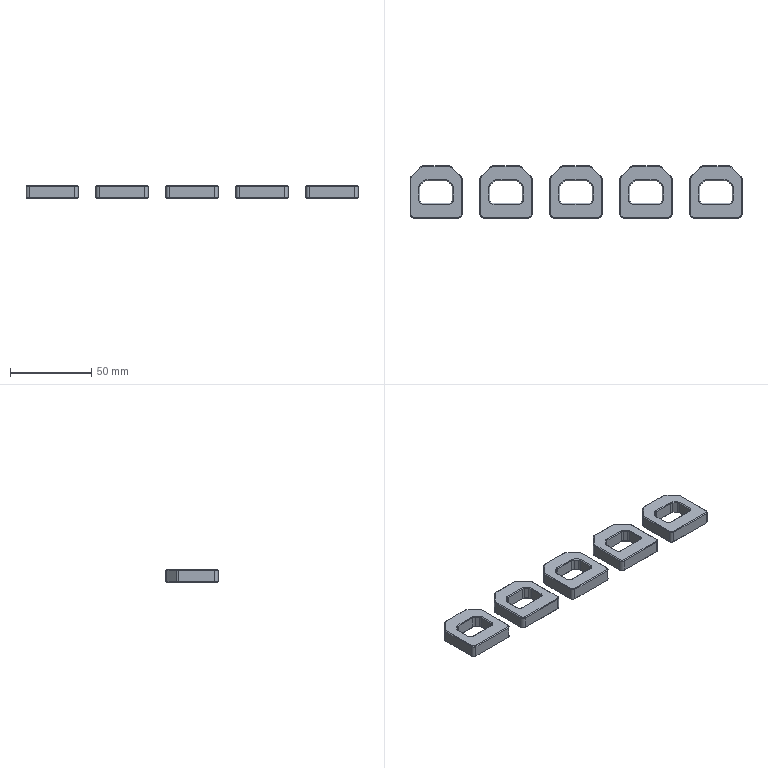NC program | NX | posted with a generic post | part box 204 x 32 x 8 mm
Lines 3721 to 4691 of 9506:
(ZLEVEL_PROFILE_COPY_1_COPY_1 , TOOL : D4)
N7428 T11 M6
N7430 G54
N7432 G17 G0 G90 X90.741 Y-4.7 S9500 M3
N7434 G43 Z30. H11
N7436 Z-0.4
N7438 G94 G1 X90.857 Y-4.9 F1000.
N7440 G3 X91.203 Y-5.1 R0.4
N7442 G1 X94. F1800.
N7444 X94.065 Y-5.113
N7446 X94.113 Y-5.065
N7448 X94.1 Y-5.
N7450 Y-2.203
N7452 G3 X93.9 Y-1.857 R0.4
N7454 G1 X93.7 Y-1.741
N7456 G0 X90.641 Y-4.6 Z-0.8
N7458 G1 X90.757 Y-4.8 F1000.
N7460 G3 X91.103 Y-5. R0.4
N7462 G1 X94. F1800.
N7464 Y-4.867
N7466 Y-2.103
N7468 G3 X93.8 Y-1.757 R0.4
N7470 G1 X93.6 Y-1.641
N7472 G0 X90.641 Y-4.6 Z-1.2
N7474 G1 X90.757 Y-4.8 F1000.
N7476 G3 X91.103 Y-5. R0.4
N7478 G1 X94. F1800.
N7480 Y-4.867
N7482 Y-2.103
N7484 G3 X93.8 Y-1.757 R0.4
N7486 G1 X93.6 Y-1.641
N7488 G0 X90.641 Y-4.6 Z-1.6
N7490 G1 X90.757 Y-4.8 F1000.
N7492 G3 X91.103 Y-5. R0.4
N7494 G1 X94. F1800.
N7496 Y-4.867
N7498 Y-2.103
N7500 G3 X93.8 Y-1.757 R0.4
N7502 G1 X93.6 Y-1.641
N7504 G0 X90.641 Y-4.6 Z-2.
N7506 G1 X90.757 Y-4.8 F1000.
N7508 G3 X91.103 Y-5. R0.4
N7510 G1 X94. F1800.
N7512 Y-4.867
N7514 Y-2.103
N7516 G3 X93.8 Y-1.757 R0.4
N7518 G1 X93.6 Y-1.641
N7520 G0 X90.641 Y-4.6 Z-2.4
N7522 G1 X90.757 Y-4.8 F1000.
N7524 G3 X91.103 Y-5. R0.4
N7526 G1 X94. F1800.
N7528 Y-4.867
N7530 Y-2.103
N7532 G3 X93.8 Y-1.757 R0.4
N7534 G1 X93.6 Y-1.641
N7536 G0 X90.641 Y-4.6 Z-2.8
N7538 G1 X90.757 Y-4.8 F1000.
N7540 G3 X91.103 Y-5. R0.4
N7542 G1 X94. F1800.
N7544 Y-4.867
N7546 Y-2.103
N7548 G3 X93.8 Y-1.757 R0.4
N7550 G1 X93.6 Y-1.641
N7552 G0 X90.641 Y-4.6 Z-3.2
N7554 G1 X90.757 Y-4.8 F1000.
N7556 G3 X91.103 Y-5. R0.4
N7558 G1 X94. F1800.
N7560 Y-4.867
N7562 Y-2.103
N7564 G3 X93.8 Y-1.757 R0.4
N7566 G1 X93.6 Y-1.641
N7568 G0 X90.641 Y-4.6 Z-3.6
N7570 G1 X90.757 Y-4.8 F1000.
N7572 G3 X91.103 Y-5. R0.4
N7574 G1 X94. F1800.
N7576 Y-4.867
N7578 Y-2.103
N7580 G3 X93.8 Y-1.757 R0.4
N7582 G1 X93.6 Y-1.641
N7584 G0 X90.641 Y-4.6 Z-4.
N7586 G1 X90.757 Y-4.8 F1000.
N7588 G3 X91.103 Y-5. R0.4
N7590 G1 X94. F1800.
N7592 Y-4.867
N7594 Y-2.103
N7596 G3 X93.8 Y-1.757 R0.4
N7598 G1 X93.6 Y-1.641
N7600 G0 X90.641 Y-4.6 Z-4.4
N7602 G1 X90.757 Y-4.8 F1000.
N7604 G3 X91.103 Y-5. R0.4
N7606 G1 X94. F1800.
N7608 Y-4.867
N7610 Y-2.103
N7612 G3 X93.8 Y-1.757 R0.4
N7614 G1 X93.6 Y-1.641
N7616 G0 X90.641 Y-4.6 Z-4.8
N7618 G1 X90.757 Y-4.8 F1000.
N7620 G3 X91.103 Y-5. R0.4
N7622 G1 X94. F1800.
N7624 Y-4.867
N7626 Y-2.103
N7628 G3 X93.8 Y-1.757 R0.4
N7630 G1 X93.6 Y-1.641
N7632 G0 X90.641 Y-4.6 Z-5.2
N7634 G1 X90.757 Y-4.8 F1000.
N7636 G3 X91.103 Y-5. R0.4
N7638 G1 X94. F1800.
N7640 Y-4.867
N7642 Y-2.103
N7644 G3 X93.8 Y-1.757 R0.4
N7646 G1 X93.6 Y-1.641
N7648 G0 X90.641 Y-4.6 Z-5.6
N7650 G1 X90.757 Y-4.8 F1000.
N7652 G3 X91.103 Y-5. R0.4
N7654 G1 X94. F1800.
N7656 Y-4.867
N7658 Y-2.103
N7660 G3 X93.8 Y-1.757 R0.4
N7662 G1 X93.6 Y-1.641
N7664 G0 X90.641 Y-4.6 Z-6.
N7666 G1 X90.757 Y-4.8 F1000.
N7668 G3 X91.103 Y-5. R0.4
N7670 G1 X94. F1800.
N7672 Y-4.867
N7674 Y-2.103
N7676 G3 X93.8 Y-1.757 R0.4
N7678 G1 X93.6 Y-1.641
N7680 G0 X90.641 Y-4.6 Z-6.4
N7682 G1 X90.757 Y-4.8 F1000.
N7684 G3 X91.103 Y-5. R0.4
N7686 G1 X94. F1800.
N7688 Y-4.867
N7690 Y-2.103
N7692 G3 X93.8 Y-1.757 R0.4
N7694 G1 X93.6 Y-1.641
N7696 G0 X90.641 Y-4.6 Z-6.8
N7698 G1 X90.757 Y-4.8 F1000.
N7700 G3 X91.103 Y-5. R0.4
N7702 G1 X94. F1800.
N7704 Y-4.867
N7706 Y-2.103
N7708 G3 X93.8 Y-1.757 R0.4
N7710 G1 X93.6 Y-1.641
N7712 G0 X90.641 Y-4.6 Z-7.2
N7714 G1 X90.757 Y-4.8 F1000.
N7716 G3 X91.103 Y-5. R0.4
N7718 G1 X94. F1800.
N7720 Y-4.867
N7722 Y-2.103
N7724 G3 X93.8 Y-1.757 R0.4
N7726 G1 X93.6 Y-1.641
N7728 G0 X90.639 Y-4.6 Z-7.6
N7730 G1 X90.754 Y-4.8 F1000.
N7732 G3 X91.101 Y-5. R0.4
N7734 G1 X94. F1800.
N7736 Y-4.867
N7738 Y-2.103
N7740 G3 X93.8 Y-1.756 R0.4
N7742 G1 X93.6 Y-1.641
N7744 G0 X90.639 Y-4.6 Z-8.
N7746 G1 X90.754 Y-4.8 F1000.
N7748 G3 X91.101 Y-5. R0.4
N7750 G1 X94. F1800.
N7752 Y-4.867
N7754 Y-2.103
N7756 G3 X93.8 Y-1.756 R0.4
N7758 G1 X93.6 Y-1.641
N7760 G0 Z30.
N7762 X93.7 Y1.611
N7764 Z-0.4
N7766 G1 X93.9 Y1.727 F1000.
N7768 G3 X94.1 Y2.073 R0.4
N7770 G1 Y3.172 F1800.
N7772 X94.12 Y3.221
N7774 X94.071 Y3.242
N7776 X93.294 Y4.019
N7778 G3 X92.908 Y4.122 R0.4
N7780 G1 X92.685 Y4.063
N7782 G0 X93.6 Y1.57 Z-0.8
N7784 G1 X93.8 Y1.685 F1000.
N7786 G3 X94. Y2.032 R0.4
N7788 G1 Y3.172 F1800.
N7790 X93.194 Y3.978
N7792 G3 X92.808 Y4.081 R0.4
N7794 G1 X92.585 Y4.021
N7796 G0 X93.6 Y1.57 Z-1.2
N7798 G1 X93.8 Y1.685 F1000.
N7800 G3 X94. Y2.032 R0.4
N7802 G1 Y3.172 F1800.
N7804 X93.194 Y3.978
N7806 G3 X92.808 Y4.081 R0.4
N7808 G1 X92.585 Y4.021
N7810 G0 X93.6 Y1.57 Z-1.6
N7812 G1 X93.8 Y1.685 F1000.
N7814 G3 X94. Y2.032 R0.4
N7816 G1 Y3.172 F1800.
N7818 X93.194 Y3.978
N7820 G3 X92.808 Y4.081 R0.4
N7822 G1 X92.585 Y4.021
N7824 G0 X93.6 Y1.57 Z-2.
N7826 G1 X93.8 Y1.685 F1000.
N7828 G3 X94. Y2.032 R0.4
N7830 G1 Y3.172 F1800.
N7832 X93.194 Y3.978
N7834 G3 X92.808 Y4.081 R0.4
N7836 G1 X92.585 Y4.021
N7838 G0 X93.6 Y1.57 Z-2.4
N7840 G1 X93.8 Y1.685 F1000.
N7842 G3 X94. Y2.032 R0.4
N7844 G1 Y3.172 F1800.
N7846 X93.194 Y3.978
N7848 G3 X92.808 Y4.081 R0.4
N7850 G1 X92.585 Y4.021
N7852 G0 X93.6 Y1.57 Z-2.8
N7854 G1 X93.8 Y1.685 F1000.
N7856 G3 X94. Y2.032 R0.4
N7858 G1 Y3.172 F1800.
N7860 X93.194 Y3.978
N7862 G3 X92.808 Y4.081 R0.4
N7864 G1 X92.585 Y4.021
N7866 G0 X93.6 Y1.57 Z-3.2
N7868 G1 X93.8 Y1.685 F1000.
N7870 G3 X94. Y2.032 R0.4
N7872 G1 Y3.172 F1800.
N7874 X93.194 Y3.978
N7876 G3 X92.808 Y4.081 R0.4
N7878 G1 X92.585 Y4.021
N7880 G0 X93.6 Y1.57 Z-3.6
N7882 G1 X93.8 Y1.685 F1000.
N7884 G3 X94. Y2.032 R0.4
N7886 G1 Y3.172 F1800.
N7888 X93.194 Y3.978
N7890 G3 X92.808 Y4.081 R0.4
N7892 G1 X92.585 Y4.021
N7894 G0 X93.6 Y1.57 Z-4.
N7896 G1 X93.8 Y1.685 F1000.
N7898 G3 X94. Y2.032 R0.4
N7900 G1 Y3.172 F1800.
N7902 X93.194 Y3.978
N7904 G3 X92.808 Y4.081 R0.4
N7906 G1 X92.585 Y4.021
N7908 G0 X93.6 Y1.57 Z-4.4
N7910 G1 X93.8 Y1.685 F1000.
N7912 G3 X94. Y2.032 R0.4
N7914 G1 Y3.172 F1800.
N7916 X93.194 Y3.978
N7918 G3 X92.808 Y4.081 R0.4
N7920 G1 X92.585 Y4.021
N7922 G0 X93.6 Y1.57 Z-4.8
N7924 G1 X93.8 Y1.685 F1000.
N7926 G3 X94. Y2.032 R0.4
N7928 G1 Y3.172 F1800.
N7930 X93.194 Y3.978
N7932 G3 X92.808 Y4.081 R0.4
N7934 G1 X92.585 Y4.021
N7936 G0 X93.6 Y1.57 Z-5.2
N7938 G1 X93.8 Y1.685 F1000.
N7940 G3 X94. Y2.032 R0.4
N7942 G1 Y3.172 F1800.
N7944 X93.194 Y3.978
N7946 G3 X92.808 Y4.081 R0.4
N7948 G1 X92.585 Y4.021
N7950 G0 X93.6 Y1.57 Z-5.6
N7952 G1 X93.8 Y1.685 F1000.
N7954 G3 X94. Y2.032 R0.4
N7956 G1 Y3.172 F1800.
N7958 X93.194 Y3.978
N7960 G3 X92.808 Y4.081 R0.4
N7962 G1 X92.585 Y4.021
N7964 G0 X93.6 Y1.57 Z-6.
N7966 G1 X93.8 Y1.685 F1000.
N7968 G3 X94. Y2.032 R0.4
N7970 G1 Y3.172 F1800.
N7972 X93.194 Y3.978
N7974 G3 X92.808 Y4.081 R0.4
N7976 G1 X92.585 Y4.021
N7978 G0 X93.6 Y1.57 Z-6.4
N7980 G1 X93.8 Y1.685 F1000.
N7982 G3 X94. Y2.032 R0.4
N7984 G1 Y3.172 F1800.
N7986 X93.194 Y3.978
N7988 G3 X92.808 Y4.081 R0.4
N7990 G1 X92.585 Y4.021
N7992 G0 X93.6 Y1.57 Z-6.8
N7994 G1 X93.8 Y1.685 F1000.
N7996 G3 X94. Y2.032 R0.4
N7998 G1 Y3.172 F1800.
N8000 X93.194 Y3.978
N8002 G3 X92.808 Y4.081 R0.4
N8004 G1 X92.585 Y4.021
N8006 G0 X93.6 Y1.57 Z-7.2
N8008 G1 X93.8 Y1.685 F1000.
N8010 G3 X94. Y2.032 R0.4
N8012 G1 Y3.172 F1800.
N8014 X93.194 Y3.978
N8016 G3 X92.808 Y4.081 R0.4
N8018 G1 X92.585 Y4.021
N8020 G0 X93.6 Y1.572 Z-7.6
N8022 G1 X93.8 Y1.688 F1000.
N8024 G3 X94. Y2.034 R0.4
N8026 G1 Y3.172 F1800.
N8028 X93.196 Y3.976
N8030 G3 X92.809 Y4.079 R0.4
N8032 G1 X92.586 Y4.02
N8034 G0 X93.6 Y1.572 Z-8.
N8036 G1 X93.8 Y1.688 F1000.
N8038 G3 X94. Y2.034 R0.4
N8040 G1 Y3.172 F1800.
N8042 X93.196 Y3.976
N8044 G3 X92.809 Y4.079 R0.4
N8046 G1 X92.586 Y4.02
N8048 G0 Z30.
N8050 X93.063 Y3.685
N8052 Z-0.4
N8054 G1 X93.122 Y3.908 F1000.
N8056 G3 X93.019 Y4.294 R0.4
N8058 G1 X92.242 Y5.071 F1800.
N8060 X92.221 Y5.12
N8062 X92.172 Y5.1
N8064 X91.073
N8066 G3 X90.727 Y4.9 R0.4
N8068 G1 X90.611 Y4.7
N8070 G0 X93.021 Y3.585 Z-0.8
N8072 G1 X93.081 Y3.808 F1000.
N8074 G3 X92.977 Y4.194 R0.4
N8076 G1 X92.171 Y5. F1800.
N8078 X91.032
N8080 G3 X90.686 Y4.8 R0.4
N8082 G1 X90.57 Y4.6
N8084 G0 X93.021 Y3.585 Z-1.2
N8086 G1 X93.081 Y3.808 F1000.
N8088 G3 X92.977 Y4.194 R0.4
N8090 G1 X92.171 Y5. F1800.
N8092 X91.032
N8094 G3 X90.686 Y4.8 R0.4
N8096 G1 X90.57 Y4.6
N8098 G0 X93.021 Y3.585 Z-1.6
N8100 G1 X93.081 Y3.808 F1000.
N8102 G3 X92.977 Y4.194 R0.4
N8104 G1 X92.171 Y5. F1800.
N8106 X91.032
N8108 G3 X90.686 Y4.8 R0.4
N8110 G1 X90.57 Y4.6
N8112 G0 X93.021 Y3.585 Z-2.
N8114 G1 X93.081 Y3.808 F1000.
N8116 G3 X92.977 Y4.194 R0.4
N8118 G1 X92.171 Y5. F1800.
N8120 X91.032
N8122 G3 X90.686 Y4.8 R0.4
N8124 G1 X90.57 Y4.6
N8126 G0 X93.021 Y3.585 Z-2.4
N8128 G1 X93.081 Y3.808 F1000.
N8130 G3 X92.977 Y4.194 R0.4
N8132 G1 X92.171 Y5. F1800.
N8134 X91.032
N8136 G3 X90.686 Y4.8 R0.4
N8138 G1 X90.57 Y4.6
N8140 G0 X93.021 Y3.585 Z-2.8
N8142 G1 X93.081 Y3.808 F1000.
N8144 G3 X92.977 Y4.194 R0.4
N8146 G1 X92.171 Y5. F1800.
N8148 X91.032
N8150 G3 X90.686 Y4.8 R0.4
N8152 G1 X90.57 Y4.6
N8154 G0 X93.021 Y3.585 Z-3.2
N8156 G1 X93.081 Y3.808 F1000.
N8158 G3 X92.977 Y4.194 R0.4
N8160 G1 X92.171 Y5. F1800.
N8162 X91.032
N8164 G3 X90.686 Y4.8 R0.4
N8166 G1 X90.57 Y4.6
N8168 G0 X93.021 Y3.585 Z-3.6
N8170 G1 X93.081 Y3.808 F1000.
N8172 G3 X92.977 Y4.194 R0.4
N8174 G1 X92.171 Y5. F1800.
N8176 X91.032
N8178 G3 X90.686 Y4.8 R0.4
N8180 G1 X90.57 Y4.6
N8182 G0 X93.021 Y3.585 Z-4.
N8184 G1 X93.081 Y3.808 F1000.
N8186 G3 X92.977 Y4.194 R0.4
N8188 G1 X92.171 Y5. F1800.
N8190 X91.032
N8192 G3 X90.686 Y4.8 R0.4
N8194 G1 X90.57 Y4.6
N8196 G0 X93.021 Y3.585 Z-4.4
N8198 G1 X93.081 Y3.808 F1000.
N8200 G3 X92.977 Y4.194 R0.4
N8202 G1 X92.171 Y5. F1800.
N8204 X91.032
N8206 G3 X90.686 Y4.8 R0.4
N8208 G1 X90.57 Y4.6
N8210 G0 X93.021 Y3.585 Z-4.8
N8212 G1 X93.081 Y3.808 F1000.
N8214 G3 X92.977 Y4.194 R0.4
N8216 G1 X92.171 Y5. F1800.
N8218 X91.032
N8220 G3 X90.686 Y4.8 R0.4
N8222 G1 X90.57 Y4.6
N8224 G0 X93.021 Y3.585 Z-5.2
N8226 G1 X93.081 Y3.808 F1000.
N8228 G3 X92.977 Y4.194 R0.4
N8230 G1 X92.171 Y5. F1800.
N8232 X91.032
N8234 G3 X90.686 Y4.8 R0.4
N8236 G1 X90.57 Y4.6
N8238 G0 X93.021 Y3.585 Z-5.6
N8240 G1 X93.081 Y3.808 F1000.
N8242 G3 X92.977 Y4.194 R0.4
N8244 G1 X92.171 Y5. F1800.
N8246 X91.032
N8248 G3 X90.686 Y4.8 R0.4
N8250 G1 X90.57 Y4.6
N8252 G0 X93.021 Y3.585 Z-6.
N8254 G1 X93.081 Y3.808 F1000.
N8256 G3 X92.977 Y4.194 R0.4
N8258 G1 X92.171 Y5. F1800.
N8260 X91.032
N8262 G3 X90.686 Y4.8 R0.4
N8264 G1 X90.57 Y4.6
N8266 G0 X93.021 Y3.585 Z-6.4
N8268 G1 X93.081 Y3.808 F1000.
N8270 G3 X92.977 Y4.194 R0.4
N8272 G1 X92.171 Y5. F1800.
N8274 X91.032
N8276 G3 X90.686 Y4.8 R0.4
N8278 G1 X90.57 Y4.6
N8280 G0 X93.021 Y3.585 Z-6.8
N8282 G1 X93.081 Y3.808 F1000.
N8284 G3 X92.977 Y4.194 R0.4
N8286 G1 X92.171 Y5. F1800.
N8288 X91.032
N8290 G3 X90.686 Y4.8 R0.4
N8292 G1 X90.57 Y4.6
N8294 G0 X93.021 Y3.585 Z-7.2
N8296 G1 X93.081 Y3.808 F1000.
N8298 G3 X92.977 Y4.194 R0.4
N8300 G1 X92.171 Y5. F1800.
N8302 X91.032
N8304 G3 X90.686 Y4.8 R0.4
N8306 G1 X90.57 Y4.6
N8308 G0 X93.007 Y3.599 Z-7.6
N8310 G1 X93.066 Y3.822 F1000.
N8312 G3 X92.963 Y4.209 R0.4
N8314 G1 X92.172 Y5. F1800.
N8316 X91.05
N8318 G3 X90.703 Y4.8 R0.4
N8320 G1 X90.588 Y4.6
N8322 G0 X93.007 Y3.599 Z-8.
N8324 G1 X93.066 Y3.822 F1000.
N8326 G3 X92.963 Y4.209 R0.4
N8328 G1 X92.172 Y5. F1800.
N8330 X91.05
N8332 G3 X90.703 Y4.8 R0.4
N8334 G1 X90.588 Y4.6
N8336 G0 Z30.
N8338 X81.389 Y4.7
N8340 Z-0.4
N8342 G1 X81.273 Y4.9 F1000.
N8344 G3 X80.927 Y5.1 R0.4
N8346 G1 X79.828 F1800.
N8348 X79.779 Y5.12
N8350 X79.758 Y5.071
N8352 X78.981 Y4.294
N8354 G3 X78.878 Y3.908 R0.4
N8356 G1 X78.937 Y3.685
N8358 G0 X81.43 Y4.6 Z-0.8
N8360 G1 X81.314 Y4.8 F1000.
N8362 G3 X80.968 Y5. R0.4
N8364 G1 X79.828 F1800.
N8366 X79.023 Y4.194
N8368 G3 X78.919 Y3.808 R0.4
N8370 G1 X78.979 Y3.585
N8372 G0 X81.43 Y4.6 Z-1.2
N8374 G1 X81.314 Y4.8 F1000.
N8376 G3 X80.968 Y5. R0.4
N8378 G1 X79.828 F1800.
N8380 X79.023 Y4.194
N8382 G3 X78.919 Y3.808 R0.4
N8384 G1 X78.979 Y3.585
N8386 G0 X81.43 Y4.6 Z-1.6
N8388 G1 X81.314 Y4.8 F1000.
N8390 G3 X80.968 Y5. R0.4
N8392 G1 X79.828 F1800.
N8394 X79.023 Y4.194
N8396 G3 X78.919 Y3.808 R0.4
N8398 G1 X78.979 Y3.585
N8400 G0 X81.43 Y4.6 Z-2.
N8402 G1 X81.314 Y4.8 F1000.
N8404 G3 X80.968 Y5. R0.4
N8406 G1 X79.828 F1800.
N8408 X79.023 Y4.194
N8410 G3 X78.919 Y3.808 R0.4
N8412 G1 X78.979 Y3.585
N8414 G0 X81.43 Y4.6 Z-2.4
N8416 G1 X81.314 Y4.8 F1000.
N8418 G3 X80.968 Y5. R0.4
N8420 G1 X79.828 F1800.
N8422 X79.023 Y4.194
N8424 G3 X78.919 Y3.808 R0.4
N8426 G1 X78.979 Y3.585
N8428 G0 X81.43 Y4.6 Z-2.8
N8430 G1 X81.314 Y4.8 F1000.
N8432 G3 X80.968 Y5. R0.4
N8434 G1 X79.828 F1800.
N8436 X79.023 Y4.194
N8438 G3 X78.919 Y3.808 R0.4
N8440 G1 X78.979 Y3.585
N8442 G0 X81.43 Y4.6 Z-3.2
N8444 G1 X81.314 Y4.8 F1000.
N8446 G3 X80.968 Y5. R0.4
N8448 G1 X79.828 F1800.
N8450 X79.023 Y4.194
N8452 G3 X78.919 Y3.808 R0.4
N8454 G1 X78.979 Y3.585
N8456 G0 X81.43 Y4.6 Z-3.6
N8458 G1 X81.314 Y4.8 F1000.
N8460 G3 X80.968 Y5. R0.4
N8462 G1 X79.828 F1800.
N8464 X79.023 Y4.194
N8466 G3 X78.919 Y3.808 R0.4
N8468 G1 X78.979 Y3.585
N8470 G0 X81.43 Y4.6 Z-4.
N8472 G1 X81.314 Y4.8 F1000.
N8474 G3 X80.968 Y5. R0.4
N8476 G1 X79.828 F1800.
N8478 X79.023 Y4.194
N8480 G3 X78.919 Y3.808 R0.4
N8482 G1 X78.979 Y3.585
N8484 G0 X81.43 Y4.6 Z-4.4
N8486 G1 X81.314 Y4.8 F1000.
N8488 G3 X80.968 Y5. R0.4
N8490 G1 X79.828 F1800.
N8492 X79.023 Y4.194
N8494 G3 X78.919 Y3.808 R0.4
N8496 G1 X78.979 Y3.585
N8498 G0 X81.43 Y4.6 Z-4.8
N8500 G1 X81.314 Y4.8 F1000.
N8502 G3 X80.968 Y5. R0.4
N8504 G1 X79.828 F1800.
N8506 X79.023 Y4.194
N8508 G3 X78.919 Y3.808 R0.4
N8510 G1 X78.979 Y3.585
N8512 G0 X81.43 Y4.6 Z-5.2
N8514 G1 X81.314 Y4.8 F1000.
N8516 G3 X80.968 Y5. R0.4
N8518 G1 X79.828 F1800.
N8520 X79.023 Y4.194
N8522 G3 X78.919 Y3.808 R0.4
N8524 G1 X78.979 Y3.585
N8526 G0 X81.43 Y4.6 Z-5.6
N8528 G1 X81.314 Y4.8 F1000.
N8530 G3 X80.968 Y5. R0.4
N8532 G1 X79.828 F1800.
N8534 X79.023 Y4.194
N8536 G3 X78.919 Y3.808 R0.4
N8538 G1 X78.979 Y3.585
N8540 G0 X81.43 Y4.6 Z-6.
N8542 G1 X81.314 Y4.8 F1000.
N8544 G3 X80.968 Y5. R0.4
N8546 G1 X79.828 F1800.
N8548 X79.023 Y4.194
N8550 G3 X78.919 Y3.808 R0.4
N8552 G1 X78.979 Y3.585
N8554 G0 X81.43 Y4.6 Z-6.4
N8556 G1 X81.314 Y4.8 F1000.
N8558 G3 X80.968 Y5. R0.4
N8560 G1 X79.828 F1800.
N8562 X79.023 Y4.194
N8564 G3 X78.919 Y3.808 R0.4
N8566 G1 X78.979 Y3.585
N8568 G0 X81.43 Y4.6 Z-6.8
N8570 G1 X81.314 Y4.8 F1000.
N8572 G3 X80.968 Y5. R0.4
N8574 G1 X79.828 F1800.
N8576 X79.023 Y4.194
N8578 G3 X78.919 Y3.808 R0.4
N8580 G1 X78.979 Y3.585
N8582 G0 X81.43 Y4.6 Z-7.2
N8584 G1 X81.314 Y4.8 F1000.
N8586 G3 X80.968 Y5. R0.4
N8588 G1 X79.828 F1800.
N8590 X79.023 Y4.194
N8592 G3 X78.919 Y3.808 R0.4
N8594 G1 X78.979 Y3.585
N8596 G0 X81.427 Y4.6 Z-7.6
N8598 G1 X81.311 Y4.8 F1000.
N8600 G3 X80.965 Y5. R0.4
N8602 G1 X79.828 F1800.
N8604 X79.029 Y4.201
N8606 G3 X78.926 Y3.814 R0.4
N8608 G1 X78.985 Y3.591
N8610 G0 X81.427 Y4.6 Z-8.
N8612 G1 X81.311 Y4.8 F1000.
N8614 G3 X80.965 Y5. R0.4
N8616 G1 X79.828 F1800.
N8618 X79.029 Y4.201
N8620 G3 X78.926 Y3.814 R0.4
N8622 G1 X78.985 Y3.591
N8624 G0 Z30.
N8626 X79.315 Y4.063
N8628 Z-0.4
N8630 G1 X79.092 Y4.122 F1000.
N8632 G3 X78.706 Y4.019 R0.4
N8634 G1 X77.929 Y3.242 F1800.
N8636 X77.88 Y3.221
N8638 X77.9 Y3.172
N8640 Y2.073
N8642 G3 X78.1 Y1.727 R0.4
N8644 G1 X78.3 Y1.611
N8646 G0 X79.415 Y4.021 Z-0.8
N8648 G1 X79.192 Y4.081 F1000.
N8650 G3 X78.806 Y3.977 R0.4
N8652 G1 X78. Y3.172 F1800.
N8654 Y2.032
N8656 G3 X78.2 Y1.686 R0.4
N8658 G1 X78.4 Y1.57
N8660 G0 X79.415 Y4.021 Z-1.2
N8662 G1 X79.192 Y4.081 F1000.
N8664 G3 X78.806 Y3.977 R0.4
N8666 G1 X78. Y3.172 F1800.
N8668 Y2.032
N8670 G3 X78.2 Y1.686 R0.4
N8672 G1 X78.4 Y1.57
N8674 G0 X79.415 Y4.021 Z-1.6
N8676 G1 X79.192 Y4.081 F1000.
N8678 G3 X78.806 Y3.977 R0.4
N8680 G1 X78. Y3.172 F1800.
N8682 Y2.032
N8684 G3 X78.2 Y1.686 R0.4
N8686 G1 X78.4 Y1.57
N8688 G0 X79.415 Y4.021 Z-2.
N8690 G1 X79.192 Y4.081 F1000.
N8692 G3 X78.806 Y3.977 R0.4
N8694 G1 X78. Y3.172 F1800.
N8696 Y2.032
N8698 G3 X78.2 Y1.686 R0.4
N8700 G1 X78.4 Y1.57
N8702 G0 X79.415 Y4.021 Z-2.4
N8704 G1 X79.192 Y4.081 F1000.
N8706 G3 X78.806 Y3.977 R0.4
N8708 G1 X78. Y3.172 F1800.
N8710 Y2.032
N8712 G3 X78.2 Y1.686 R0.4
N8714 G1 X78.4 Y1.57
N8716 G0 X79.415 Y4.021 Z-2.8
N8718 G1 X79.192 Y4.081 F1000.
N8720 G3 X78.806 Y3.977 R0.4
N8722 G1 X78. Y3.172 F1800.
N8724 Y2.032
N8726 G3 X78.2 Y1.686 R0.4
N8728 G1 X78.4 Y1.57
N8730 G0 X79.415 Y4.021 Z-3.2
N8732 G1 X79.192 Y4.081 F1000.
N8734 G3 X78.806 Y3.977 R0.4
N8736 G1 X78. Y3.172 F1800.
N8738 Y2.032
N8740 G3 X78.2 Y1.686 R0.4
N8742 G1 X78.4 Y1.57
N8744 G0 X79.415 Y4.021 Z-3.6
N8746 G1 X79.192 Y4.081 F1000.
N8748 G3 X78.806 Y3.977 R0.4
N8750 G1 X78. Y3.172 F1800.
N8752 Y2.032
N8754 G3 X78.2 Y1.686 R0.4
N8756 G1 X78.4 Y1.57
N8758 G0 X79.415 Y4.021 Z-4.
N8760 G1 X79.192 Y4.081 F1000.
N8762 G3 X78.806 Y3.977 R0.4
N8764 G1 X78. Y3.172 F1800.
N8766 Y2.032
N8768 G3 X78.2 Y1.686 R0.4
N8770 G1 X78.4 Y1.57
N8772 G0 X79.415 Y4.021 Z-4.4
N8774 G1 X79.192 Y4.081 F1000.
N8776 G3 X78.806 Y3.977 R0.4
N8778 G1 X78. Y3.172 F1800.
N8780 Y2.032
N8782 G3 X78.2 Y1.686 R0.4
N8784 G1 X78.4 Y1.57
N8786 G0 X79.415 Y4.021 Z-4.8
N8788 G1 X79.192 Y4.081 F1000.
N8790 G3 X78.806 Y3.977 R0.4
N8792 G1 X78. Y3.172 F1800.
N8794 Y2.032
N8796 G3 X78.2 Y1.686 R0.4
N8798 G1 X78.4 Y1.57
N8800 G0 X79.415 Y4.021 Z-5.2
N8802 G1 X79.192 Y4.081 F1000.
N8804 G3 X78.806 Y3.977 R0.4
N8806 G1 X78. Y3.172 F1800.
N8808 Y2.032
N8810 G3 X78.2 Y1.686 R0.4
N8812 G1 X78.4 Y1.57
N8814 G0 X79.415 Y4.021 Z-5.6
N8816 G1 X79.192 Y4.081 F1000.
N8818 G3 X78.806 Y3.977 R0.4
N8820 G1 X78. Y3.172 F1800.
N8822 Y2.032
N8824 G3 X78.2 Y1.686 R0.4
N8826 G1 X78.4 Y1.57
N8828 G0 X79.415 Y4.021 Z-6.
N8830 G1 X79.192 Y4.081 F1000.
N8832 G3 X78.806 Y3.977 R0.4
N8834 G1 X78. Y3.172 F1800.
N8836 Y2.032
N8838 G3 X78.2 Y1.686 R0.4
N8840 G1 X78.4 Y1.57
N8842 G0 X79.415 Y4.021 Z-6.4
N8844 G1 X79.192 Y4.081 F1000.
N8846 G3 X78.806 Y3.977 R0.4
N8848 G1 X78. Y3.172 F1800.
N8850 Y2.032
N8852 G3 X78.2 Y1.686 R0.4
N8854 G1 X78.4 Y1.57
N8856 G0 X79.415 Y4.021 Z-6.8
N8858 G1 X79.192 Y4.081 F1000.
N8860 G3 X78.806 Y3.977 R0.4
N8862 G1 X78. Y3.172 F1800.
N8864 Y2.032
N8866 G3 X78.2 Y1.686 R0.4
N8868 G1 X78.4 Y1.57
N8870 G0 X79.415 Y4.021 Z-7.2
N8872 G1 X79.192 Y4.081 F1000.
N8874 G3 X78.806 Y3.977 R0.4
N8876 G1 X78. Y3.172 F1800.
N8878 Y2.032
N8880 G3 X78.2 Y1.686 R0.4
N8882 G1 X78.4 Y1.57
N8884 G0 X79.402 Y4.008 Z-7.6
N8886 G1 X79.179 Y4.068 F1000.
N8888 G3 X78.793 Y3.964 R0.4
N8890 G1 X78. Y3.172 F1800.
N8892 Y2.048
N8894 G3 X78.2 Y1.702 R0.4
N8896 G1 X78.4 Y1.586
N8898 G0 X79.402 Y4.008 Z-8.
N8900 G1 X79.179 Y4.068 F1000.
N8902 G3 X78.793 Y3.964 R0.4
N8904 G1 X78. Y3.172 F1800.
N8906 Y2.048
N8908 G3 X78.2 Y1.702 R0.4
N8910 G1 X78.4 Y1.586
N8912 G0 Z30.
N8914 X78.3 Y-1.741
N8916 Z-0.4
N8918 G1 X78.1 Y-1.857 F1000.
N8920 G3 X77.9 Y-2.203 R0.4
N8922 G1 Y-5. F1800.
N8924 X77.887 Y-5.065
N8926 X77.935 Y-5.113
N8928 X78. Y-5.1
N8930 X80.797
N8932 G3 X81.143 Y-4.9 R0.4
N8934 G1 X81.259 Y-4.7
N8936 G0 X78.4 Y-1.641 Z-0.8
N8938 G1 X78.2 Y-1.757 F1000.
N8940 G3 X78. Y-2.103 R0.4
N8942 G1 Y-4.87 F1800.
N8944 X77.997 Y-5.003
N8946 X78.042 Y-5.
N8948 X80.897
N8950 G3 X81.243 Y-4.8 R0.4
N8952 G1 X81.359 Y-4.6
N8954 G0 X78.4 Y-1.641 Z-1.2
N8956 G1 X78.2 Y-1.757 F1000.
N8958 G3 X78. Y-2.103 R0.4
N8960 G1 Y-4.87 F1800.
N8962 X77.997 Y-5.003
N8964 X78.042 Y-5.
N8966 X80.897
N8968 G3 X81.243 Y-4.8 R0.4
N8970 G1 X81.359 Y-4.6
N8972 G0 X78.4 Y-1.641 Z-1.6
N8974 G1 X78.2 Y-1.757 F1000.
N8976 G3 X78. Y-2.103 R0.4
N8978 G1 Y-4.87 F1800.
N8980 X77.997 Y-5.003
N8982 X80.897 Y-5.
N8984 G3 X81.243 Y-4.8 R0.4
N8986 G1 X81.359 Y-4.6
N8988 G0 X78.4 Y-1.641 Z-2.
N8990 G1 X78.2 Y-1.757 F1000.
N8992 G3 X78. Y-2.103 R0.4
N8994 G1 Y-4.87 F1800.
N8996 X77.997 Y-5.003
N8998 X80.897 Y-5.
N9000 G3 X81.243 Y-4.8 R0.4
N9002 G1 X81.359 Y-4.6
N9004 G0 X78.4 Y-1.641 Z-2.4
N9006 G1 X78.2 Y-1.757 F1000.
N9008 G3 X78. Y-2.103 R0.4
N9010 G1 Y-4.87 F1800.
N9012 X77.997 Y-5.003
N9014 X80.897 Y-5.
N9016 G3 X81.243 Y-4.8 R0.4
N9018 G1 X81.359 Y-4.6
N9020 G0 X78.4 Y-1.641 Z-2.8
N9022 G1 X78.2 Y-1.757 F1000.
N9024 G3 X78. Y-2.103 R0.4
N9026 G1 Y-4.87 F1800.
N9028 X77.998 Y-5.002
N9030 X80.897 Y-5.
N9032 G3 X81.243 Y-4.8 R0.4
N9034 G1 X81.359 Y-4.6
N9036 G0 X78.4 Y-1.641 Z-3.2
N9038 G1 X78.2 Y-1.757 F1000.
N9040 G3 X78. Y-2.103 R0.4
N9042 G1 Y-4.87 F1800.
N9044 X77.998 Y-5.002
N9046 X80.897 Y-5.
N9048 G3 X81.243 Y-4.8 R0.4
N9050 G1 X81.359 Y-4.6
N9052 G0 X78.4 Y-1.641 Z-3.6
N9054 G1 X78.2 Y-1.757 F1000.
N9056 G3 X78. Y-2.103 R0.4
N9058 G1 Y-4.87 F1800.
N9060 X77.998 Y-5.002
N9062 X80.897 Y-5.
N9064 G3 X81.243 Y-4.8 R0.4
N9066 G1 X81.359 Y-4.6
N9068 G0 X78.4 Y-1.641 Z-4.
N9070 G1 X78.2 Y-1.757 F1000.
N9072 G3 X78. Y-2.103 R0.4
N9074 G1 Y-4.87 F1800.
N9076 X77.998 Y-5.002
N9078 X80.897 Y-5.
N9080 G3 X81.243 Y-4.8 R0.4
N9082 G1 X81.359 Y-4.6
N9084 G0 X78.4 Y-1.641 Z-4.4
N9086 G1 X78.2 Y-1.757 F1000.
N9088 G3 X78. Y-2.103 R0.4
N9090 G1 Y-4.87 F1800.
N9092 X77.998 Y-5.002
N9094 X80.897 Y-5.
N9096 G3 X81.243 Y-4.8 R0.4
N9098 G1 X81.359 Y-4.6
N9100 G0 X78.4 Y-1.641 Z-4.8
N9102 G1 X78.2 Y-1.757 F1000.
N9104 G3 X78. Y-2.103 R0.4
N9106 G1 Y-4.87 F1800.
N9108 X77.998 Y-5.002
N9110 X80.897 Y-5.
N9112 G3 X81.243 Y-4.8 R0.4
N9114 G1 X81.359 Y-4.6
N9116 G0 X78.4 Y-1.641 Z-5.2
N9118 G1 X78.2 Y-1.757 F1000.
N9120 G3 X78. Y-2.103 R0.4
N9122 G1 Y-4.87 F1800.
N9124 X77.999 Y-5.001
N9126 X80.897 Y-5.
N9128 G3 X81.243 Y-4.8 R0.4
N9130 G1 X81.359 Y-4.6
N9132 G0 X78.4 Y-1.641 Z-5.6
N9134 G1 X78.2 Y-1.757 F1000.
N9136 G3 X78. Y-2.103 R0.4
N9138 G1 Y-4.87 F1800.
N9140 X77.999 Y-5.001
N9142 X80.897 Y-5.
N9144 G3 X81.243 Y-4.8 R0.4
N9146 G1 X81.359 Y-4.6
N9148 G0 X78.4 Y-1.641 Z-6.
N9150 G1 X78.2 Y-1.757 F1000.
N9152 G3 X78. Y-2.103 R0.4
N9154 G1 Y-4.87 F1800.
N9156 X77.999 Y-5.001
N9158 X80.897 Y-5.
N9160 G3 X81.243 Y-4.8 R0.4
N9162 G1 X81.359 Y-4.6
N9164 G0 X78.4 Y-1.641 Z-6.4
N9166 G1 X78.2 Y-1.757 F1000.
N9168 G3 X78. Y-2.103 R0.4
N9170 G1 Y-4.87 F1800.
N9172 X77.999 Y-5.001
N9174 X80.897 Y-5.
N9176 G3 X81.243 Y-4.8 R0.4
N9178 G1 X81.359 Y-4.6
N9180 G0 X78.4 Y-1.641 Z-6.8
N9182 G1 X78.2 Y-1.757 F1000.
N9184 G3 X78. Y-2.103 R0.4
N9186 G1 Y-4.87 F1800.
N9188 X77.999 Y-5.001
N9190 X80.897 Y-5.
N9192 G3 X81.243 Y-4.8 R0.4
N9194 G1 X81.359 Y-4.6
N9196 G0 X78.4 Y-1.641 Z-7.2
N9198 G1 X78.2 Y-1.757 F1000.
N9200 G3 X78. Y-2.103 R0.4
N9202 G1 Y-4.87 F1800.
N9204 X77.999 Y-5.001
N9206 X80.897 Y-5.
N9208 G3 X81.243 Y-4.8 R0.4
N9210 G1 X81.359 Y-4.6
N9212 G0 X78.4 Y-1.641 Z-7.6
N9214 G1 X78.2 Y-1.757 F1000.
N9216 G3 X78. Y-2.103 R0.4
N9218 G1 Y-4.87 F1800.
N9220 Y-5.
N9222 X80.897
N9224 G3 X81.243 Y-4.8 R0.4
N9226 G1 X81.359 Y-4.6
N9228 G0 X78.4 Y-1.641 Z-8.
N9230 G1 X78.2 Y-1.757 F1000.
N9232 G3 X78. Y-2.103 R0.4
N9234 G1 Y-4.87 F1800.
N9236 Y-5.
N9238 X80.897
N9240 G3 X81.243 Y-4.8 R0.4
N9242 G1 X81.359 Y-4.6
N9244 G0 Z30.
N9246 X-7.7 Y-1.741
N9248 Z-0.4
N9250 G1 X-7.9 Y-1.857 F1000.
N9252 G3 X-8.1 Y-2.203 R0.4
N9254 G1 Y-5. F1800.
N9256 X-8.113 Y-5.065
N9258 X-8.065 Y-5.113
N9260 X-8. Y-5.1
N9262 X-5.203
N9264 G3 X-4.857 Y-4.9 R0.4
N9266 G1 X-4.741 Y-4.7
N9268 G0 X-7.6 Y-1.641 Z-0.8
N9270 G1 X-7.8 Y-1.757 F1000.
N9272 G3 X-8. Y-2.103 R0.4
N9274 G1 Y-4.87 F1800.
N9276 X-8.002 Y-5.002
N9278 X-5.103 Y-5.
N9280 G3 X-4.757 Y-4.8 R0.4
N9282 G1 X-4.641 Y-4.6
N9284 G0 X-7.6 Y-1.641 Z-1.2
N9286 G1 X-7.8 Y-1.757 F1000.
N9288 G3 X-8. Y-2.103 R0.4
N9290 G1 Y-4.87 F1800.
N9292 X-8.002 Y-5.002
N9294 X-5.103 Y-5.
N9296 G3 X-4.757 Y-4.8 R0.4
N9298 G1 X-4.641 Y-4.6
N9300 G0 X-7.6 Y-1.641 Z-1.6
N9302 G1 X-7.8 Y-1.757 F1000.
N9304 G3 X-8. Y-2.103 R0.4
N9306 G1 Y-4.87 F1800.
N9308 X-8.002 Y-5.002
N9310 X-5.103 Y-5.
N9312 G3 X-4.757 Y-4.8 R0.4
N9314 G1 X-4.641 Y-4.6
N9316 G0 X-7.6 Y-1.641 Z-2.
N9318 G1 X-7.8 Y-1.757 F1000.
N9320 G3 X-8. Y-2.103 R0.4
N9322 G1 Y-4.87 F1800.
N9324 X-8.002 Y-5.002
N9326 X-5.103 Y-5.
N9328 G3 X-4.757 Y-4.8 R0.4
N9330 G1 X-4.641 Y-4.6
N9332 G0 X-7.6 Y-1.641 Z-2.4
N9334 G1 X-7.8 Y-1.757 F1000.
N9336 G3 X-8. Y-2.103 R0.4
N9338 G1 Y-4.87 F1800.
N9340 X-8.001 Y-5.001
N9342 X-5.103 Y-5.
N9344 G3 X-4.757 Y-4.8 R0.4
N9346 G1 X-4.641 Y-4.6
N9348 G0 X-7.6 Y-1.641 Z-2.8
N9350 G1 X-7.8 Y-1.757 F1000.
N9352 G3 X-8. Y-2.103 R0.4
N9354 G1 Y-4.87 F1800.
N9356 X-8.001 Y-5.001
N9358 X-5.103 Y-5.
N9360 G3 X-4.757 Y-4.8 R0.4
N9362 G1 X-4.641 Y-4.6